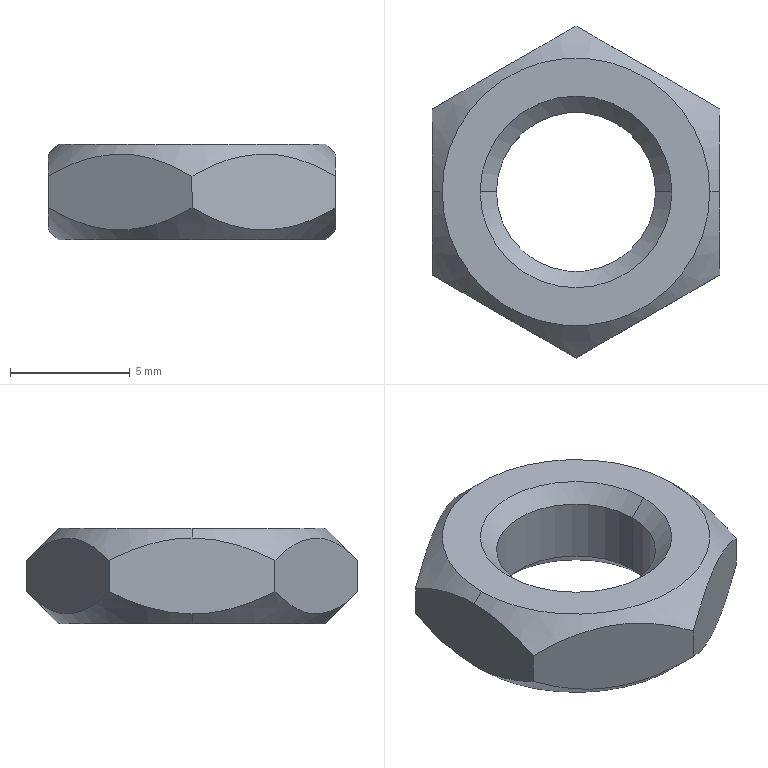Part | STEP file | PN_0032 | 1 solid | 18 faces | box 12 x 13.856 x 4 mm | volume 327.385 mm3 | cone 8 | plane 8 | cylinder 2 | commonest cylinder face diameters 6.647 x2